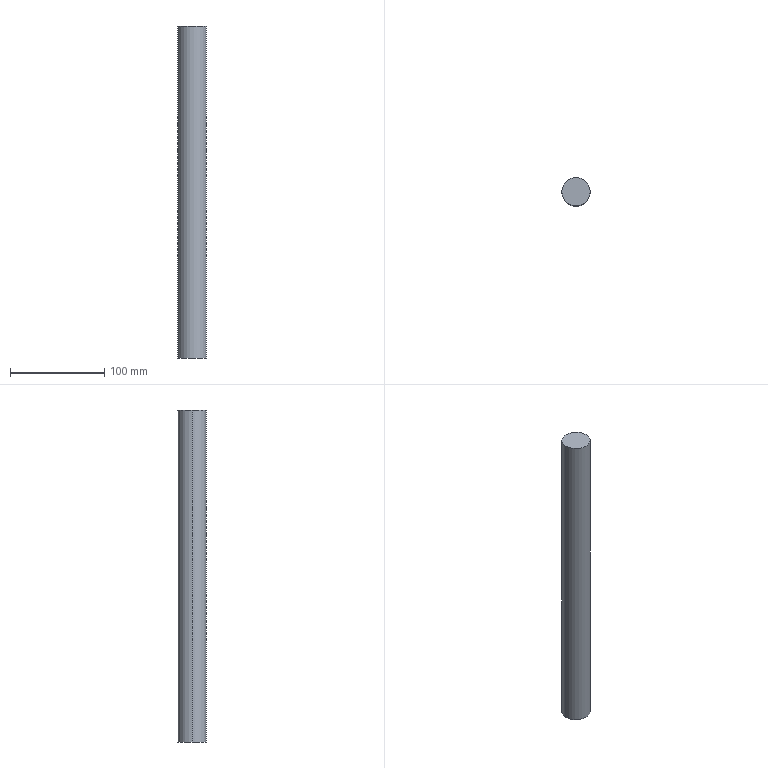Part | SolidWorks | features Extrusion 1, ICE 1 | 1 solid | 4 faces | box 30 x 30 x 352 mm | volume 248814 mm3 | cylinder 2 | plane 2 | commonest cylinder face diameters 30 x2
STEP:
#1=CARTESIAN_POINT('',(15.,0.,352.));
#2=VERTEX_POINT('',#1);
#3=CARTESIAN_POINT('',(-15.,0.,352.));
#4=VERTEX_POINT('',#3);
#5=CARTESIAN_POINT('',(0.,0.,352.));
#6=DIRECTION('',(0.,0.,1.));
#7=DIRECTION('',(1.,0.,0.));
#8=AXIS2_PLACEMENT_3D('',#5,#6,#7);
#9=CIRCLE('',#8,15.);
#10=EDGE_CURVE('',#2,#4,#9,.T.);
#11=ORIENTED_EDGE('',*,*,#10,.F.);
#12=CARTESIAN_POINT('',(15.,0.,0.));
#13=VERTEX_POINT('',#12);
#14=CARTESIAN_POINT('',(15.,0.,400.));
#15=DIRECTION('',(0.,0.,-1.));
#16=VECTOR('',#15,1000.);
#17=LINE('',#14,#16);
#18=EDGE_CURVE('',#2,#13,#17,.T.);
#19=ORIENTED_EDGE('',*,*,#18,.T.);
#20=CARTESIAN_POINT('',(-15.,0.,0.));
#21=VERTEX_POINT('',#20);
#22=CARTESIAN_POINT('',(0.,0.,0.));
#23=DIRECTION('',(0.,0.,1.));
#24=DIRECTION('',(1.,0.,0.));
#25=AXIS2_PLACEMENT_3D('',#22,#23,#24);
#26=CIRCLE('',#25,15.);
#27=EDGE_CURVE('',#13,#21,#26,.T.);
#28=ORIENTED_EDGE('',*,*,#27,.T.);
#29=CARTESIAN_POINT('',(-15.,0.,400.));
#30=DIRECTION('',(0.,0.,-1.));
#31=VECTOR('',#30,1000.);
#32=LINE('',#29,#31);
#33=EDGE_CURVE('',#4,#21,#32,.T.);
#34=ORIENTED_EDGE('',*,*,#33,.F.);
#35=EDGE_LOOP('',(#11,#19,#28,#34));
#36=FACE_OUTER_BOUND('',#35,.T.);
#37=CARTESIAN_POINT('',(0.,0.,400.));
#38=DIRECTION('',(0.,0.,-1.));
#39=DIRECTION('',(-1.,0.,0.));
#40=AXIS2_PLACEMENT_3D('',#37,#38,#39);
#41=CYLINDRICAL_SURFACE('',#40,15.);
#42=ADVANCED_FACE('',(#36),#41,.T.);
#43=ORIENTED_EDGE('',*,*,#18,.F.);
#44=CARTESIAN_POINT('',(0.,0.,352.));
#45=DIRECTION('',(0.,0.,1.));
#46=DIRECTION('',(1.,0.,0.));
#47=AXIS2_PLACEMENT_3D('',#44,#45,#46);
#48=CIRCLE('',#47,15.);
#49=EDGE_CURVE('',#4,#2,#48,.T.);
#50=ORIENTED_EDGE('',*,*,#49,.F.);
#51=ORIENTED_EDGE('',*,*,#33,.T.);
#52=CARTESIAN_POINT('',(0.,0.,0.));
#53=DIRECTION('',(0.,0.,1.));
#54=DIRECTION('',(1.,0.,0.));
#55=AXIS2_PLACEMENT_3D('',#52,#53,#54);
#56=CIRCLE('',#55,15.);
#57=EDGE_CURVE('',#21,#13,#56,.T.);
#58=ORIENTED_EDGE('',*,*,#57,.T.);
#59=EDGE_LOOP('',(#43,#50,#51,#58));
#60=FACE_OUTER_BOUND('',#59,.T.);
#61=CARTESIAN_POINT('',(0.,0.,400.));
#62=DIRECTION('',(0.,0.,-1.));
#63=DIRECTION('',(-1.,0.,0.));
#64=AXIS2_PLACEMENT_3D('',#61,#62,#63);
#65=CYLINDRICAL_SURFACE('',#64,15.);
#66=ADVANCED_FACE('',(#60),#65,.T.);
#67=ORIENTED_EDGE('',*,*,#57,.F.);
#68=ORIENTED_EDGE('',*,*,#27,.F.);
#69=EDGE_LOOP('',(#67,#68));
#70=FACE_OUTER_BOUND('',#69,.T.);
#71=CARTESIAN_POINT('',(0.,0.,0.));
#72=DIRECTION('',(0.,0.,1.));
#73=DIRECTION('',(1.,0.,0.));
#74=AXIS2_PLACEMENT_3D('',#71,#72,#73);
#75=PLANE('',#74);
#76=ADVANCED_FACE('',(#70),#75,.F.);
#77=ORIENTED_EDGE('',*,*,#49,.T.);
#78=ORIENTED_EDGE('',*,*,#10,.T.);
#79=EDGE_LOOP('',(#77,#78));
#80=FACE_OUTER_BOUND('',#79,.T.);
#81=CARTESIAN_POINT('',(0.,0.,352.));
#82=DIRECTION('',(0.,0.,1.));
#83=DIRECTION('',(1.,0.,0.));
#84=AXIS2_PLACEMENT_3D('',#81,#82,#83);
#85=PLANE('',#84);
#86=ADVANCED_FACE('',(#80),#85,.T.);
#87=CLOSED_SHELL('',(#42,#66,#76,#86));
#88=MANIFOLD_SOLID_BREP('',#87);
#89=CARTESIAN_POINT('',(0.,0.,0.));
#90=DIRECTION('',(0.,0.,1.));
#91=DIRECTION('',(1.,0.,0.));
#92=AXIS2_PLACEMENT_3D('',#89,#90,#91);
#93=(LENGTH_UNIT()NAMED_UNIT(*)SI_UNIT(.MILLI.,.METRE.));
#94=UNCERTAINTY_MEASURE_WITH_UNIT(LENGTH_MEASURE(0.00001),#93,'','');
#95=(NAMED_UNIT(*)PLANE_ANGLE_UNIT()SI_UNIT($,.RADIAN.));
#96=(NAMED_UNIT(*)SI_UNIT($,.STERADIAN.)SOLID_ANGLE_UNIT());
#97=(GEOMETRIC_REPRESENTATION_CONTEXT(3)GLOBAL_UNCERTAINTY_ASSIGNED_CONTEXT((#94))GLOBAL_UNIT_ASSIGNED_CONTEXT((#93,#95,#96))REPRESENTATION_CONTEXT('',''));
#98=ADVANCED_BREP_SHAPE_REPRESENTATION('',(#88,#92),#97);